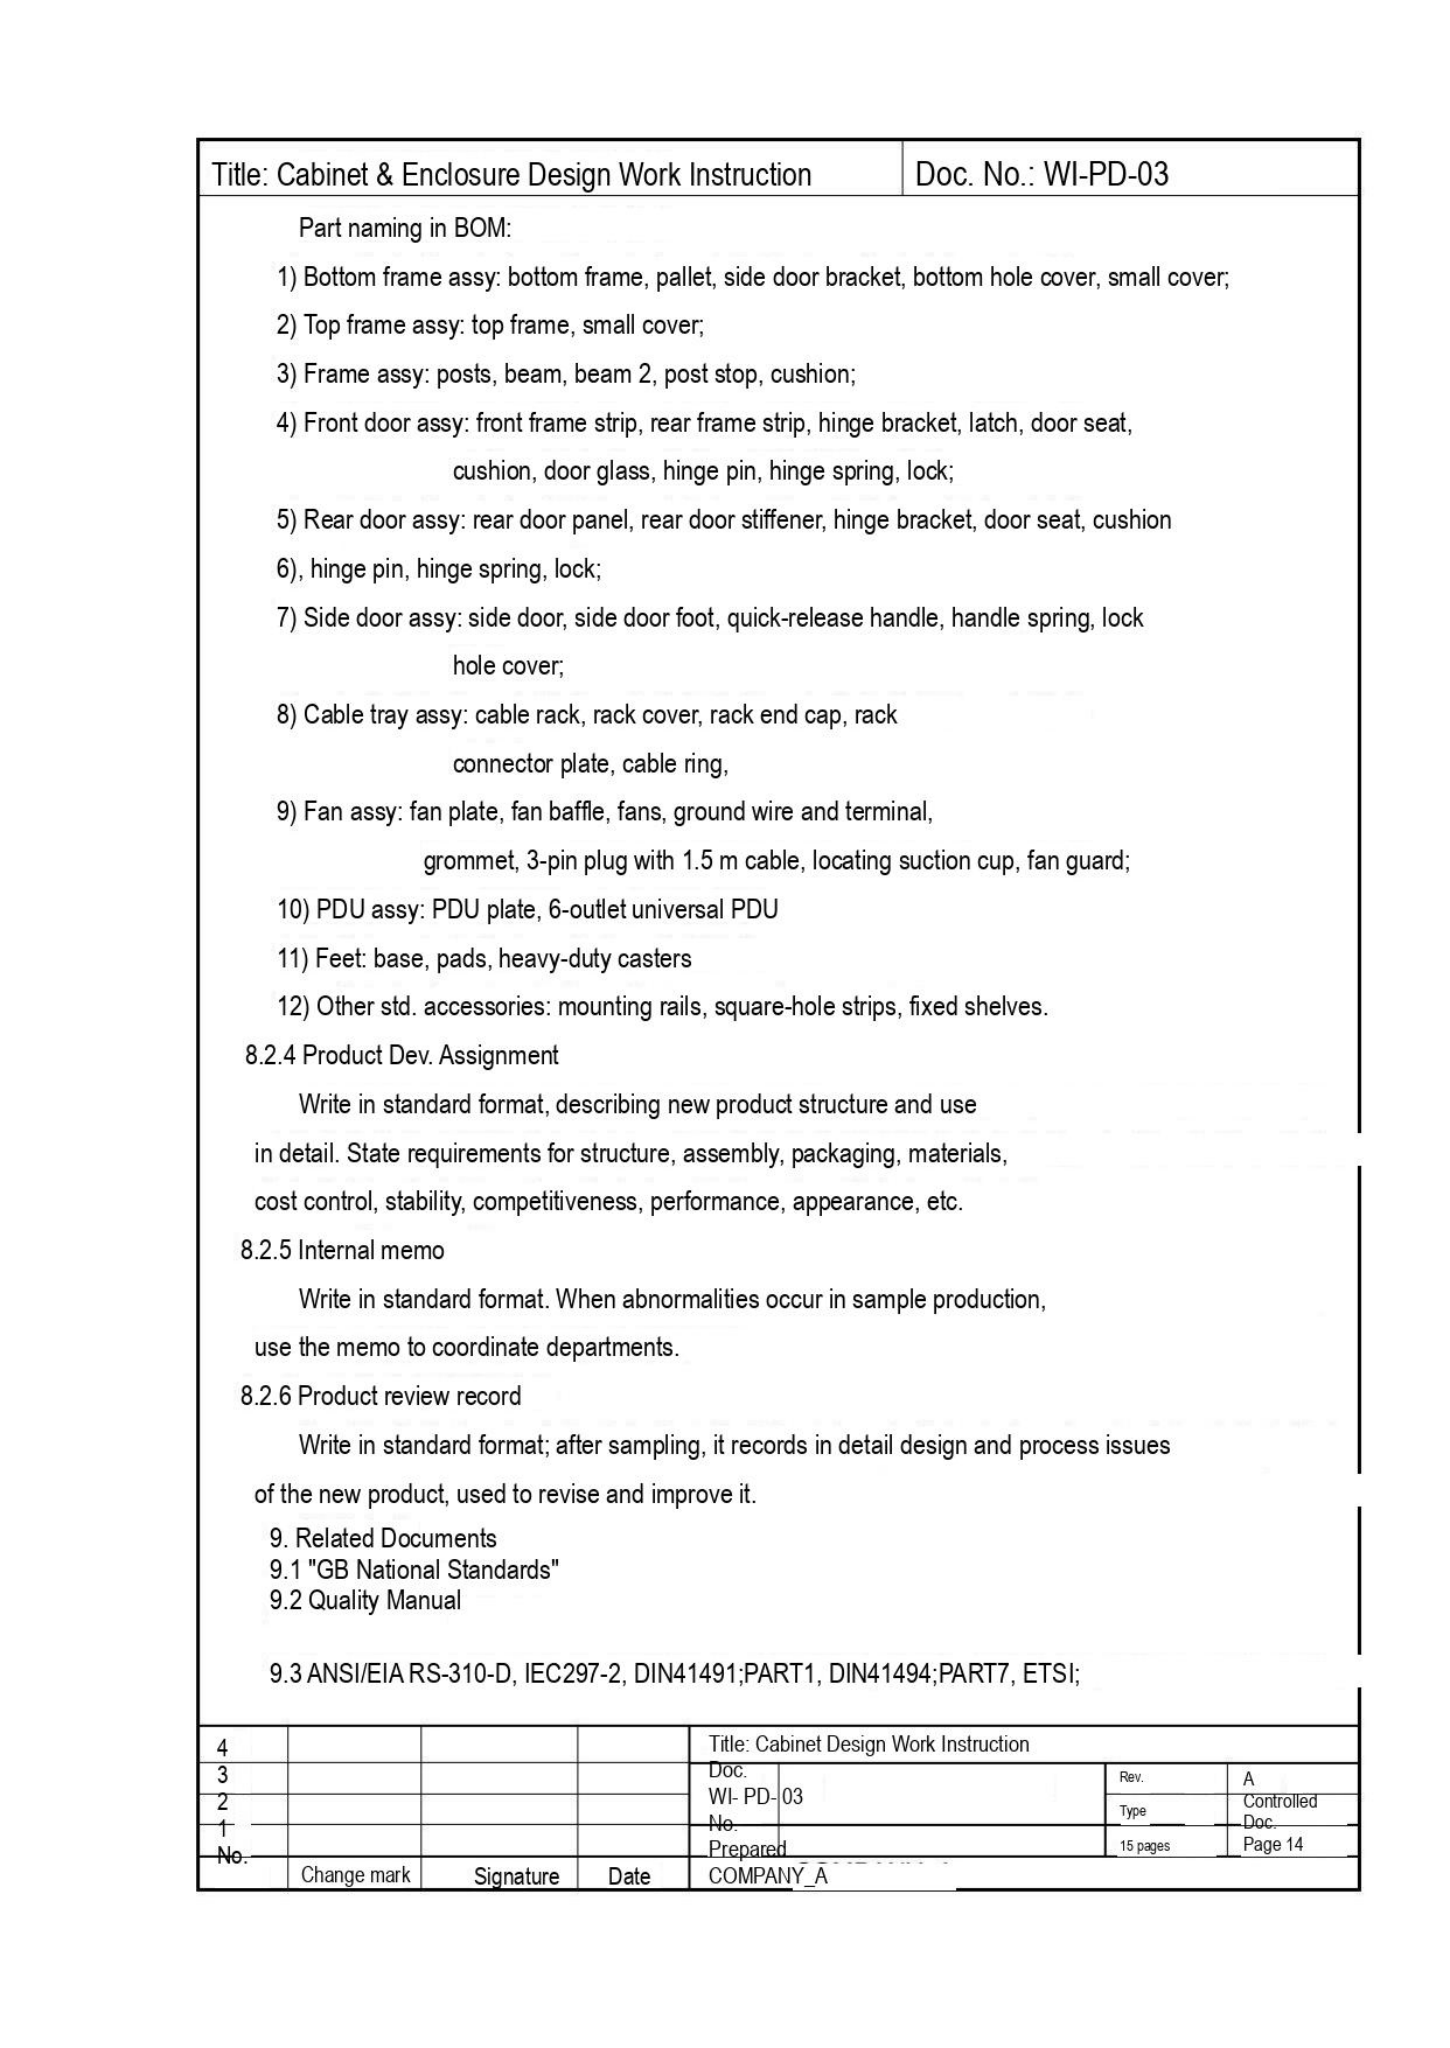Title: Cabinet & Enclosure Design Work Instruction | Doc. No.: WI-PD-03

Part naming in BOM:

1) Bottom frame assy: bottom frame, pallet, side door bracket, bottom hole cover, small cover;

2) Top frame assy: top frame, small cover;

3) Frame assy: posts, beam, beam 2, post stop, cushion;

4) Front door assy: front frame strip, rear frame strip, hinge bracket, latch, door seat, cushion, door glass, hinge pin, hinge spring, lock;

5) Rear door assy: rear door panel, rear door stiffener, hinge bracket, door seat, cushion

6), hinge pin, hinge spring, lock;

7) Side door assy: side door, side door foot, quick-release handle, handle spring, lock hole cover;

8) Cable tray assy: cable rack, rack cover, rack end cap, rack connector plate, cable ring,

9) Fan assy: fan plate, fan baffle, fans, ground wire and terminal, grommet, 3-pin plug with 1.5 m cable, locating suction cup, fan guard;

10) PDU assy: PDU plate, 6-outlet universal PDU

11) Feet: base, pads, heavy-duty casters

12) Other std. accessories: mounting rails, square-hole strips, fixed shelves.

8.2.4 Product Dev. Assignment

Write in standard format, describing new product structure and use in detail. State requirements for structure, assembly, packaging, materials, cost control, stability, competitiveness, performance, appearance, etc.

8.2.5 Internal memo

Write in standard format. When abnormalities occur in sample production, use the memo to coordinate departments.

8.2.6 Product review record

Write in standard format; after sampling, it records in detail design and process issues of the new product, used to revise and improve it.

9. Related Documents
9.1 "GB National Standards"
9.2 Quality Manual

9.3 ANSI/EIA RS-310-D, IEC297-2, DIN41491;PART1, DIN41494;PART7, ETSI;

| No. | Change mark | Signature | Date | Title: Cabinet Design Work Instruction | | |
|---|---|---|---|---|---|---|
| 4 | | | | Doc. No. WI- PD- 03 | Rev. | A |
| 3 | | | | | Type | Controlled Doc. |
| 2 | | | | | 15 pages | Page 14 |
| 1 | | | | Prepared COMPANY_A | | |
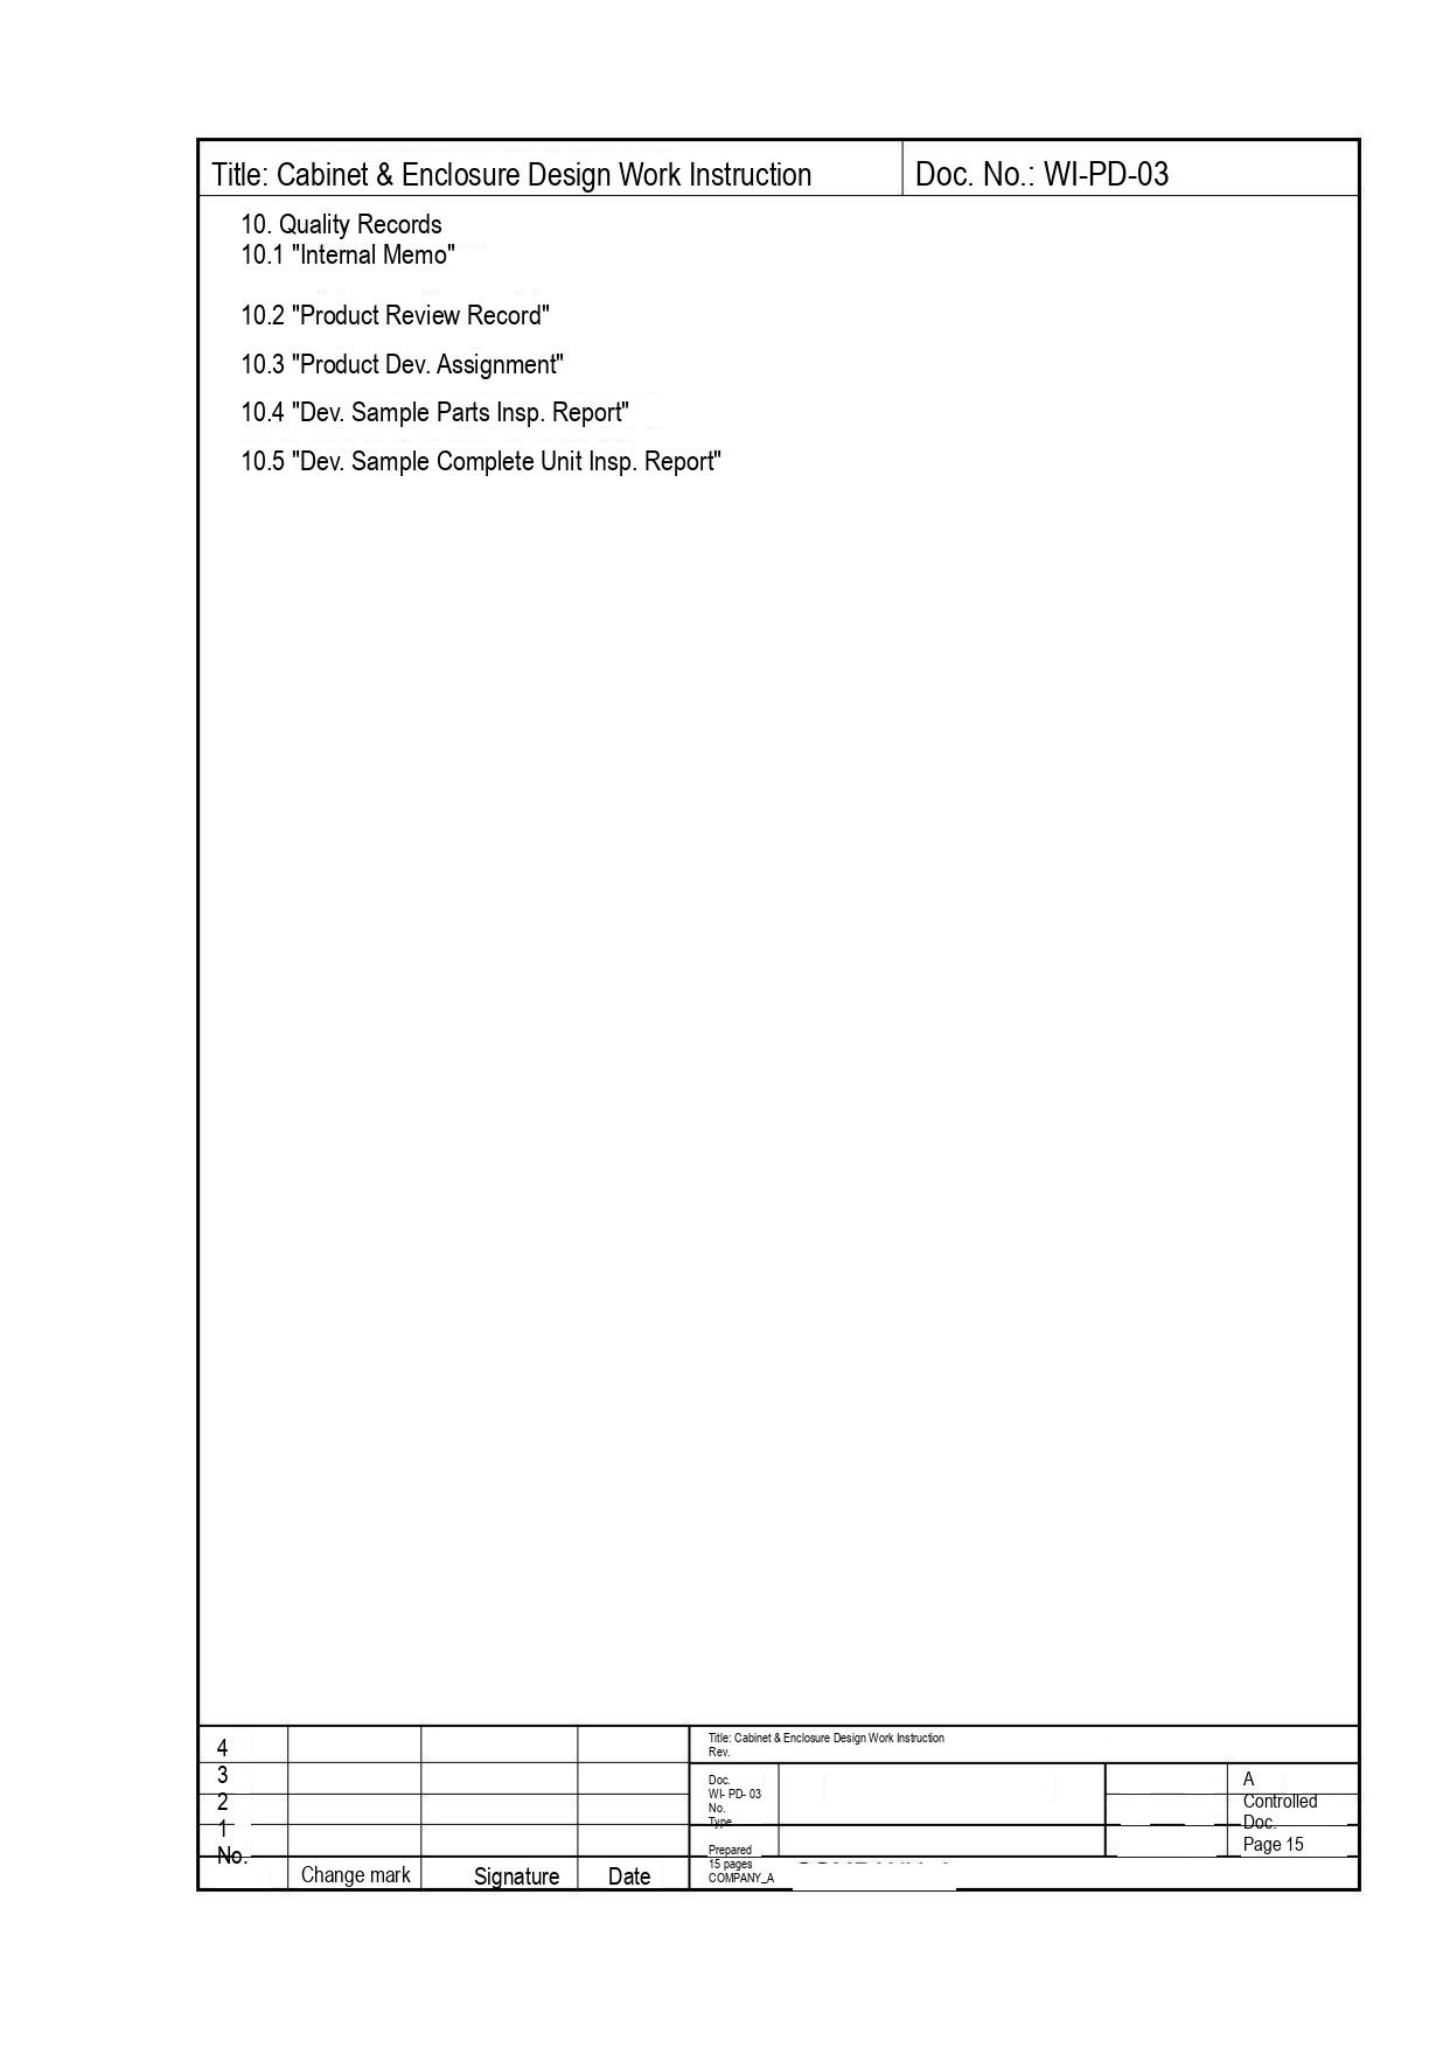| Title: Cabinet & Enclosure Design Work Instruction | Doc. No.: WI-PD-03 |
|---|---|

10. Quality Records
10.1 "Internal Memo"
10.2 "Product Review Record"
10.3 "Product Dev. Assignment"
10.4 "Dev. Sample Parts Insp. Report"
10.5 "Dev. Sample Complete Unit Insp. Report"

| No. | Change mark | Signature | Date |
|---|---|---|---|
| 4 | | | |
| 3 | | | |
| 2 | | | |
| 1 | | | |

Title: Cabinet & Enclosure Design Work Instruction
Rev.
Doc.
WI- PD- 03
No.
Type
Prepared
15 pages
COMPANY_A

A
Controlled
Doc.
Page 15